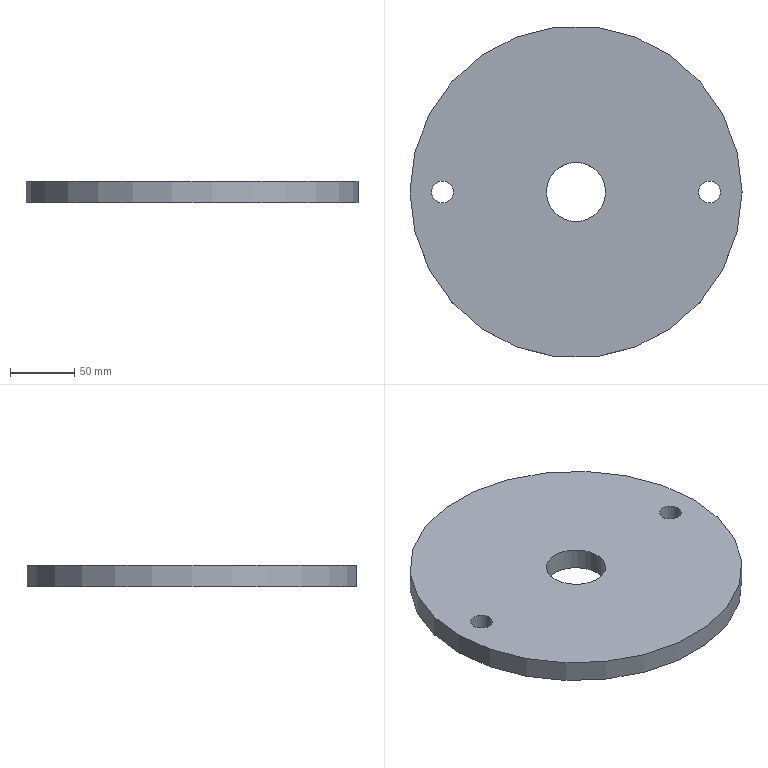Part | NX | features Delete Body 2, LINKED_BODY 2, SIMPLE HOLE 2, SYMBOLIC_THREAD 2, CYLINDER 1, DATUM_CSYS 1, MIRROR_SET 1, SCALE 1, SUBTRACT 1 | 1 solid | 6 faces | volume 851530 mm3 | cylinder 4 | plane 2 | commonest cylinder face diameters 16.948 x2 46.132 x1 258.75 x1